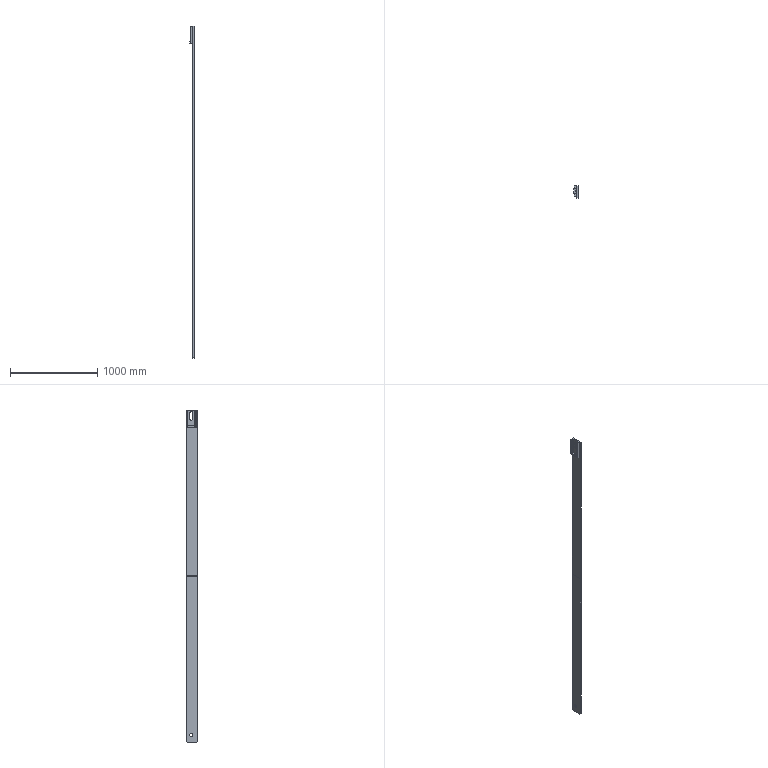Part | STEP file | 012-6-07-01-2 | 4 solids | 49 faces | box 51 x 134.1 x 3800 mm | volume 8306378 mm3 | plane 43 | cylinder 6 | commonest cylinder face diameters 12 x2 32 x2 35 x2